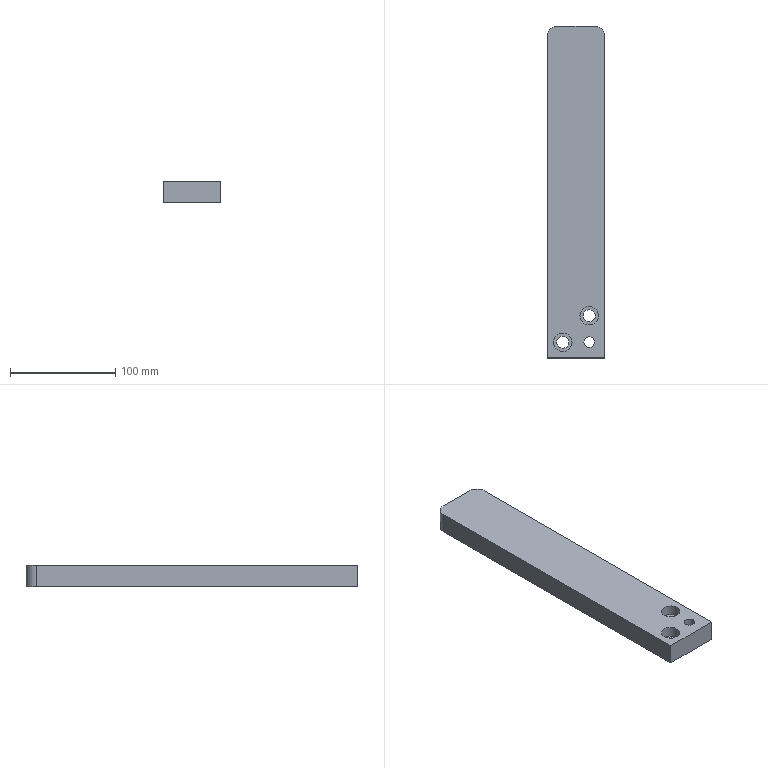Part | NX | features solid 2 | 1 solid | 15 faces | box 55 x 315 x 20 mm | volume 337183 mm3 | plane 8 | cylinder 7 | commonest cylinder face diameters 11.5 x2 17.5 x2 20 x2 10 x1
STEP:
#1=CARTESIAN_POINT('',(55.,25.,-20.));
#2=VERTEX_POINT('',#1);
#3=CARTESIAN_POINT('',(55.,25.,-40.));
#4=VERTEX_POINT('',#3);
#5=CARTESIAN_POINT('',(55.,25.,-20.));
#6=DIRECTION('',(0.,0.,-1.));
#7=VECTOR('',#6,1000.);
#8=LINE('',#5,#7);
#9=EDGE_CURVE('',#2,#4,#8,.T.);
#10=ORIENTED_EDGE('',*,*,#9,.T.);
#11=CARTESIAN_POINT('',(110.,25.,-40.));
#12=VERTEX_POINT('',#11);
#13=CARTESIAN_POINT('',(60.,25.,-40.));
#14=DIRECTION('',(-1.,0.,0.));
#15=VECTOR('',#14,1000.);
#16=LINE('',#13,#15);
#17=EDGE_CURVE('',#4,#12,#16,.F.);
#18=ORIENTED_EDGE('',*,*,#17,.T.);
#19=CARTESIAN_POINT('',(110.,25.,-20.));
#20=VERTEX_POINT('',#19);
#21=CARTESIAN_POINT('',(110.,25.,-20.));
#22=DIRECTION('',(0.,0.,1.));
#23=VECTOR('',#22,1000.);
#24=LINE('',#21,#23);
#25=EDGE_CURVE('',#20,#12,#24,.F.);
#26=ORIENTED_EDGE('',*,*,#25,.F.);
#27=CARTESIAN_POINT('',(60.,25.,-20.));
#28=DIRECTION('',(-1.,0.,0.));
#29=VECTOR('',#28,1000.);
#30=LINE('',#27,#29);
#31=EDGE_CURVE('',#2,#20,#30,.F.);
#32=ORIENTED_EDGE('',*,*,#31,.F.);
#33=EDGE_LOOP('',(#10,#18,#26,#32));
#34=FACE_BOUND('',#33,.T.);
#35=CARTESIAN_POINT('',(60.,25.,-20.));
#36=DIRECTION('',(0.,1.,0.));
#37=DIRECTION('',(1.,0.,0.));
#38=AXIS2_PLACEMENT_3D('',#35,#36,#37);
#39=PLANE('',#38);
#40=ADVANCED_FACE('',(#34),#39,.F.);
#41=CARTESIAN_POINT('',(100.,40.,-40.));
#42=VERTEX_POINT('',#41);
#43=CARTESIAN_POINT('',(95.,40.,-40.));
#44=DIRECTION('',(0.,0.,1.));
#45=DIRECTION('',(1.,0.,0.));
#46=AXIS2_PLACEMENT_3D('',#43,#44,#45);
#47=CIRCLE('',#46,5.);
#48=EDGE_CURVE('',#42,#42,#47,.T.);
#49=ORIENTED_EDGE('',*,*,#48,.T.);
#50=EDGE_LOOP('',(#49));
#51=FACE_BOUND('',#50,.T.);
#52=CARTESIAN_POINT('',(100.75,65.,-40.));
#53=VERTEX_POINT('',#52);
#54=CARTESIAN_POINT('',(95.,65.,-40.));
#55=DIRECTION('',(0.,0.,1.));
#56=DIRECTION('',(1.,0.,0.));
#57=AXIS2_PLACEMENT_3D('',#54,#55,#56);
#58=CIRCLE('',#57,5.75);
#59=EDGE_CURVE('',#53,#53,#58,.T.);
#60=ORIENTED_EDGE('',*,*,#59,.T.);
#61=EDGE_LOOP('',(#60));
#62=FACE_BOUND('',#61,.T.);
#63=CARTESIAN_POINT('',(75.75,40.,-40.));
#64=VERTEX_POINT('',#63);
#65=CARTESIAN_POINT('',(70.,40.,-40.));
#66=DIRECTION('',(0.,0.,1.));
#67=DIRECTION('',(1.,0.,0.));
#68=AXIS2_PLACEMENT_3D('',#65,#66,#67);
#69=CIRCLE('',#68,5.75);
#70=EDGE_CURVE('',#64,#64,#69,.T.);
#71=ORIENTED_EDGE('',*,*,#70,.T.);
#72=EDGE_LOOP('',(#71));
#73=FACE_BOUND('',#72,.T.);
#74=CARTESIAN_POINT('',(65.,340.,-40.));
#75=VERTEX_POINT('',#74);
#76=CARTESIAN_POINT('',(100.,340.,-40.));
#77=VERTEX_POINT('',#76);
#78=CARTESIAN_POINT('',(390.,340.,-40.));
#79=DIRECTION('',(1.,0.,0.));
#80=VECTOR('',#79,1000.);
#81=LINE('',#78,#80);
#82=EDGE_CURVE('',#75,#77,#81,.T.);
#83=ORIENTED_EDGE('',*,*,#82,.T.);
#84=CARTESIAN_POINT('',(110.,330.,-40.));
#85=VERTEX_POINT('',#84);
#86=CARTESIAN_POINT('',(100.,330.,-40.));
#87=DIRECTION('',(0.,0.,1.));
#88=DIRECTION('',(1.,0.,0.));
#89=AXIS2_PLACEMENT_3D('',#86,#87,#88);
#90=CIRCLE('',#89,10.);
#91=EDGE_CURVE('',#77,#85,#90,.F.);
#92=ORIENTED_EDGE('',*,*,#91,.T.);
#93=CARTESIAN_POINT('',(110.,120.,-40.));
#94=DIRECTION('',(0.,-1.,0.));
#95=VECTOR('',#94,1000.);
#96=LINE('',#93,#95);
#97=EDGE_CURVE('',#85,#12,#96,.T.);
#98=ORIENTED_EDGE('',*,*,#97,.T.);
#99=ORIENTED_EDGE('',*,*,#17,.F.);
#100=CARTESIAN_POINT('',(55.,330.,-40.));
#101=VERTEX_POINT('',#100);
#102=CARTESIAN_POINT('',(55.,120.,-40.));
#103=DIRECTION('',(0.,1.,0.));
#104=VECTOR('',#103,1000.);
#105=LINE('',#102,#104);
#106=EDGE_CURVE('',#101,#4,#105,.F.);
#107=ORIENTED_EDGE('',*,*,#106,.F.);
#108=CARTESIAN_POINT('',(65.,330.,-40.));
#109=DIRECTION('',(0.,0.,1.));
#110=DIRECTION('',(1.,0.,0.));
#111=AXIS2_PLACEMENT_3D('',#108,#109,#110);
#112=CIRCLE('',#111,10.);
#113=EDGE_CURVE('',#101,#75,#112,.F.);
#114=ORIENTED_EDGE('',*,*,#113,.T.);
#115=EDGE_LOOP('',(#83,#92,#98,#99,#107,#114));
#116=FACE_BOUND('',#115,.T.);
#117=CARTESIAN_POINT('',(60.,120.,-40.));
#118=DIRECTION('',(0.,0.,1.));
#119=DIRECTION('',(-1.,0.,0.));
#120=AXIS2_PLACEMENT_3D('',#117,#118,#119);
#121=PLANE('',#120);
#122=ADVANCED_FACE('',(#51,#62,#73,#116),#121,.F.);
#123=CARTESIAN_POINT('',(100.,40.,-20.));
#124=VERTEX_POINT('',#123);
#125=CARTESIAN_POINT('',(95.,40.,-20.));
#126=DIRECTION('',(0.,0.,1.));
#127=DIRECTION('',(1.,0.,0.));
#128=AXIS2_PLACEMENT_3D('',#125,#126,#127);
#129=CIRCLE('',#128,5.);
#130=EDGE_CURVE('',#124,#124,#129,.F.);
#131=ORIENTED_EDGE('',*,*,#130,.T.);
#132=EDGE_LOOP('',(#131));
#133=FACE_BOUND('',#132,.T.);
#134=CARTESIAN_POINT('',(103.75,65.,-20.));
#135=VERTEX_POINT('',#134);
#136=CARTESIAN_POINT('',(95.,65.,-20.));
#137=DIRECTION('',(0.,0.,1.));
#138=DIRECTION('',(1.,0.,0.));
#139=AXIS2_PLACEMENT_3D('',#136,#137,#138);
#140=CIRCLE('',#139,8.75);
#141=EDGE_CURVE('',#135,#135,#140,.F.);
#142=ORIENTED_EDGE('',*,*,#141,.T.);
#143=EDGE_LOOP('',(#142));
#144=FACE_BOUND('',#143,.T.);
#145=CARTESIAN_POINT('',(78.75,40.,-20.));
#146=VERTEX_POINT('',#145);
#147=CARTESIAN_POINT('',(70.,40.,-20.));
#148=DIRECTION('',(0.,0.,1.));
#149=DIRECTION('',(1.,0.,0.));
#150=AXIS2_PLACEMENT_3D('',#147,#148,#149);
#151=CIRCLE('',#150,8.75);
#152=EDGE_CURVE('',#146,#146,#151,.F.);
#153=ORIENTED_EDGE('',*,*,#152,.T.);
#154=EDGE_LOOP('',(#153));
#155=FACE_BOUND('',#154,.T.);
#156=CARTESIAN_POINT('',(110.,330.,-20.));
#157=VERTEX_POINT('',#156);
#158=CARTESIAN_POINT('',(110.,120.,-20.));
#159=DIRECTION('',(0.,-1.,0.));
#160=VECTOR('',#159,1000.);
#161=LINE('',#158,#160);
#162=EDGE_CURVE('',#157,#20,#161,.T.);
#163=ORIENTED_EDGE('',*,*,#162,.F.);
#164=CARTESIAN_POINT('',(100.,340.,-20.));
#165=VERTEX_POINT('',#164);
#166=CARTESIAN_POINT('',(100.,330.,-20.));
#167=DIRECTION('',(0.,0.,1.));
#168=DIRECTION('',(1.,0.,0.));
#169=AXIS2_PLACEMENT_3D('',#166,#167,#168);
#170=CIRCLE('',#169,10.);
#171=EDGE_CURVE('',#157,#165,#170,.T.);
#172=ORIENTED_EDGE('',*,*,#171,.T.);
#173=CARTESIAN_POINT('',(65.,340.,-20.));
#174=VERTEX_POINT('',#173);
#175=CARTESIAN_POINT('',(390.,340.,-20.));
#176=DIRECTION('',(1.,0.,0.));
#177=VECTOR('',#176,1000.);
#178=LINE('',#175,#177);
#179=EDGE_CURVE('',#174,#165,#178,.T.);
#180=ORIENTED_EDGE('',*,*,#179,.F.);
#181=CARTESIAN_POINT('',(55.,330.,-20.));
#182=VERTEX_POINT('',#181);
#183=CARTESIAN_POINT('',(65.,330.,-20.));
#184=DIRECTION('',(0.,0.,1.));
#185=DIRECTION('',(1.,0.,0.));
#186=AXIS2_PLACEMENT_3D('',#183,#184,#185);
#187=CIRCLE('',#186,10.);
#188=EDGE_CURVE('',#174,#182,#187,.T.);
#189=ORIENTED_EDGE('',*,*,#188,.T.);
#190=CARTESIAN_POINT('',(55.,120.,-20.));
#191=DIRECTION('',(0.,1.,0.));
#192=VECTOR('',#191,1000.);
#193=LINE('',#190,#192);
#194=EDGE_CURVE('',#182,#2,#193,.F.);
#195=ORIENTED_EDGE('',*,*,#194,.T.);
#196=ORIENTED_EDGE('',*,*,#31,.T.);
#197=EDGE_LOOP('',(#163,#172,#180,#189,#195,#196));
#198=FACE_BOUND('',#197,.T.);
#199=CARTESIAN_POINT('',(60.,120.,-20.));
#200=DIRECTION('',(0.,0.,1.));
#201=DIRECTION('',(-1.,0.,0.));
#202=AXIS2_PLACEMENT_3D('',#199,#200,#201);
#203=PLANE('',#202);
#204=ADVANCED_FACE('',(#133,#144,#155,#198),#203,.T.);
#205=ORIENTED_EDGE('',*,*,#97,.F.);
#206=CARTESIAN_POINT('',(110.,330.,-20.));
#207=DIRECTION('',(0.,0.,-1.));
#208=VECTOR('',#207,1000.);
#209=LINE('',#206,#208);
#210=EDGE_CURVE('',#85,#157,#209,.F.);
#211=ORIENTED_EDGE('',*,*,#210,.T.);
#212=ORIENTED_EDGE('',*,*,#162,.T.);
#213=ORIENTED_EDGE('',*,*,#25,.T.);
#214=EDGE_LOOP('',(#205,#211,#212,#213));
#215=FACE_BOUND('',#214,.T.);
#216=CARTESIAN_POINT('',(110.,120.,-20.));
#217=DIRECTION('',(1.,0.,0.));
#218=DIRECTION('',(0.,-1.,0.));
#219=AXIS2_PLACEMENT_3D('',#216,#217,#218);
#220=PLANE('',#219);
#221=ADVANCED_FACE('',(#215),#220,.T.);
#222=ORIENTED_EDGE('',*,*,#194,.F.);
#223=CARTESIAN_POINT('',(55.,330.,-20.));
#224=DIRECTION('',(0.,0.,1.));
#225=VECTOR('',#224,1000.);
#226=LINE('',#223,#225);
#227=EDGE_CURVE('',#182,#101,#226,.F.);
#228=ORIENTED_EDGE('',*,*,#227,.T.);
#229=ORIENTED_EDGE('',*,*,#106,.T.);
#230=ORIENTED_EDGE('',*,*,#9,.F.);
#231=EDGE_LOOP('',(#222,#228,#229,#230));
#232=FACE_BOUND('',#231,.T.);
#233=CARTESIAN_POINT('',(55.,120.,-20.));
#234=DIRECTION('',(1.,0.,0.));
#235=DIRECTION('',(0.,-1.,0.));
#236=AXIS2_PLACEMENT_3D('',#233,#234,#235);
#237=PLANE('',#236);
#238=ADVANCED_FACE('',(#232),#237,.F.);
#239=ORIENTED_EDGE('',*,*,#179,.T.);
#240=CARTESIAN_POINT('',(100.,340.,15.));
#241=DIRECTION('',(0.,0.,-1.));
#242=VECTOR('',#241,1000.);
#243=LINE('',#240,#242);
#244=EDGE_CURVE('',#165,#77,#243,.T.);
#245=ORIENTED_EDGE('',*,*,#244,.T.);
#246=ORIENTED_EDGE('',*,*,#82,.F.);
#247=CARTESIAN_POINT('',(65.,340.,15.));
#248=DIRECTION('',(0.,0.,-1.));
#249=VECTOR('',#248,1000.);
#250=LINE('',#247,#249);
#251=EDGE_CURVE('',#75,#174,#250,.F.);
#252=ORIENTED_EDGE('',*,*,#251,.T.);
#253=EDGE_LOOP('',(#239,#245,#246,#252));
#254=FACE_BOUND('',#253,.T.);
#255=CARTESIAN_POINT('',(390.,340.,15.));
#256=DIRECTION('',(0.,1.,0.));
#257=DIRECTION('',(0.,0.,1.));
#258=AXIS2_PLACEMENT_3D('',#255,#256,#257);
#259=PLANE('',#258);
#260=ADVANCED_FACE('',(#254),#259,.T.);
#261=CARTESIAN_POINT('',(64.25,40.,-30.));
#262=VERTEX_POINT('',#261);
#263=CARTESIAN_POINT('',(70.,40.,-30.));
#264=DIRECTION('',(0.,0.,-1.));
#265=DIRECTION('',(-1.,0.,0.));
#266=AXIS2_PLACEMENT_3D('',#263,#264,#265);
#267=CIRCLE('',#266,5.75);
#268=EDGE_CURVE('',#262,#262,#267,.T.);
#269=ORIENTED_EDGE('',*,*,#268,.F.);
#270=EDGE_LOOP('',(#269));
#271=FACE_BOUND('',#270,.T.);
#272=ORIENTED_EDGE('',*,*,#70,.F.);
#273=EDGE_LOOP('',(#272));
#274=FACE_BOUND('',#273,.T.);
#275=CARTESIAN_POINT('',(70.,40.,-115.));
#276=DIRECTION('',(0.,0.,-1.));
#277=DIRECTION('',(-1.,0.,0.));
#278=AXIS2_PLACEMENT_3D('',#275,#276,#277);
#279=CYLINDRICAL_SURFACE('',#278,5.75);
#280=ADVANCED_FACE('',(#271,#274),#279,.F.);
#281=ORIENTED_EDGE('',*,*,#268,.T.);
#282=EDGE_LOOP('',(#281));
#283=FACE_BOUND('',#282,.T.);
#284=CARTESIAN_POINT('',(61.25,40.,-30.));
#285=VERTEX_POINT('',#284);
#286=CARTESIAN_POINT('',(70.,40.,-30.));
#287=DIRECTION('',(0.,0.,-1.));
#288=DIRECTION('',(-1.,0.,0.));
#289=AXIS2_PLACEMENT_3D('',#286,#287,#288);
#290=CIRCLE('',#289,8.75);
#291=EDGE_CURVE('',#285,#285,#290,.T.);
#292=ORIENTED_EDGE('',*,*,#291,.F.);
#293=EDGE_LOOP('',(#292));
#294=FACE_BOUND('',#293,.T.);
#295=CARTESIAN_POINT('',(70.,40.,-30.));
#296=DIRECTION('',(0.,0.,-1.));
#297=DIRECTION('',(-1.,0.,0.));
#298=AXIS2_PLACEMENT_3D('',#295,#296,#297);
#299=PLANE('',#298);
#300=ADVANCED_FACE('',(#283,#294),#299,.F.);
#301=ORIENTED_EDGE('',*,*,#291,.T.);
#302=EDGE_LOOP('',(#301));
#303=FACE_BOUND('',#302,.T.);
#304=ORIENTED_EDGE('',*,*,#152,.F.);
#305=EDGE_LOOP('',(#304));
#306=FACE_BOUND('',#305,.T.);
#307=CARTESIAN_POINT('',(70.,40.,-15.));
#308=DIRECTION('',(0.,0.,-1.));
#309=DIRECTION('',(-1.,0.,0.));
#310=AXIS2_PLACEMENT_3D('',#307,#308,#309);
#311=CYLINDRICAL_SURFACE('',#310,8.75);
#312=ADVANCED_FACE('',(#303,#306),#311,.F.);
#313=CARTESIAN_POINT('',(89.25,65.,-30.));
#314=VERTEX_POINT('',#313);
#315=CARTESIAN_POINT('',(95.,65.,-30.));
#316=DIRECTION('',(0.,0.,-1.));
#317=DIRECTION('',(-1.,0.,0.));
#318=AXIS2_PLACEMENT_3D('',#315,#316,#317);
#319=CIRCLE('',#318,5.75);
#320=EDGE_CURVE('',#314,#314,#319,.T.);
#321=ORIENTED_EDGE('',*,*,#320,.F.);
#322=EDGE_LOOP('',(#321));
#323=FACE_BOUND('',#322,.T.);
#324=ORIENTED_EDGE('',*,*,#59,.F.);
#325=EDGE_LOOP('',(#324));
#326=FACE_BOUND('',#325,.T.);
#327=CARTESIAN_POINT('',(95.,65.,-115.));
#328=DIRECTION('',(0.,0.,-1.));
#329=DIRECTION('',(-1.,0.,0.));
#330=AXIS2_PLACEMENT_3D('',#327,#328,#329);
#331=CYLINDRICAL_SURFACE('',#330,5.75);
#332=ADVANCED_FACE('',(#323,#326),#331,.F.);
#333=ORIENTED_EDGE('',*,*,#320,.T.);
#334=EDGE_LOOP('',(#333));
#335=FACE_BOUND('',#334,.T.);
#336=CARTESIAN_POINT('',(86.25,65.,-30.));
#337=VERTEX_POINT('',#336);
#338=CARTESIAN_POINT('',(95.,65.,-30.));
#339=DIRECTION('',(0.,0.,-1.));
#340=DIRECTION('',(-1.,0.,0.));
#341=AXIS2_PLACEMENT_3D('',#338,#339,#340);
#342=CIRCLE('',#341,8.75);
#343=EDGE_CURVE('',#337,#337,#342,.T.);
#344=ORIENTED_EDGE('',*,*,#343,.F.);
#345=EDGE_LOOP('',(#344));
#346=FACE_BOUND('',#345,.T.);
#347=CARTESIAN_POINT('',(95.,65.,-30.));
#348=DIRECTION('',(0.,0.,-1.));
#349=DIRECTION('',(-1.,0.,0.));
#350=AXIS2_PLACEMENT_3D('',#347,#348,#349);
#351=PLANE('',#350);
#352=ADVANCED_FACE('',(#335,#346),#351,.F.);
#353=ORIENTED_EDGE('',*,*,#343,.T.);
#354=EDGE_LOOP('',(#353));
#355=FACE_BOUND('',#354,.T.);
#356=ORIENTED_EDGE('',*,*,#141,.F.);
#357=EDGE_LOOP('',(#356));
#358=FACE_BOUND('',#357,.T.);
#359=CARTESIAN_POINT('',(95.,65.,-15.));
#360=DIRECTION('',(0.,0.,-1.));
#361=DIRECTION('',(-1.,0.,0.));
#362=AXIS2_PLACEMENT_3D('',#359,#360,#361);
#363=CYLINDRICAL_SURFACE('',#362,8.75);
#364=ADVANCED_FACE('',(#355,#358),#363,.F.);
#365=ORIENTED_EDGE('',*,*,#130,.F.);
#366=EDGE_LOOP('',(#365));
#367=FACE_BOUND('',#366,.T.);
#368=ORIENTED_EDGE('',*,*,#48,.F.);
#369=EDGE_LOOP('',(#368));
#370=FACE_BOUND('',#369,.T.);
#371=CARTESIAN_POINT('',(95.,40.,-15.));
#372=DIRECTION('',(0.,0.,-1.));
#373=DIRECTION('',(-1.,0.,0.));
#374=AXIS2_PLACEMENT_3D('',#371,#372,#373);
#375=CYLINDRICAL_SURFACE('',#374,5.);
#376=ADVANCED_FACE('',(#367,#370),#375,.F.);
#377=ORIENTED_EDGE('',*,*,#171,.F.);
#378=ORIENTED_EDGE('',*,*,#210,.F.);
#379=ORIENTED_EDGE('',*,*,#91,.F.);
#380=ORIENTED_EDGE('',*,*,#244,.F.);
#381=EDGE_LOOP('',(#377,#378,#379,#380));
#382=FACE_BOUND('',#381,.T.);
#383=CARTESIAN_POINT('',(100.,330.,15.));
#384=DIRECTION('',(0.,0.,-1.));
#385=DIRECTION('',(-1.,0.,0.));
#386=AXIS2_PLACEMENT_3D('',#383,#384,#385);
#387=CYLINDRICAL_SURFACE('',#386,10.);
#388=ADVANCED_FACE('',(#382),#387,.T.);
#389=ORIENTED_EDGE('',*,*,#113,.F.);
#390=ORIENTED_EDGE('',*,*,#227,.F.);
#391=ORIENTED_EDGE('',*,*,#188,.F.);
#392=ORIENTED_EDGE('',*,*,#251,.F.);
#393=EDGE_LOOP('',(#389,#390,#391,#392));
#394=FACE_BOUND('',#393,.T.);
#395=CARTESIAN_POINT('',(65.,330.,15.));
#396=DIRECTION('',(0.,0.,-1.));
#397=DIRECTION('',(-1.,0.,0.));
#398=AXIS2_PLACEMENT_3D('',#395,#396,#397);
#399=CYLINDRICAL_SURFACE('',#398,10.);
#400=ADVANCED_FACE('',(#394),#399,.T.);
#401=CLOSED_SHELL('',(#40,#122,#204,#221,#238,#260,#280,#300,#312,#332,#352,#364,#376,#388,#400));
#402=MANIFOLD_SOLID_BREP('',#401);
#403=(LENGTH_UNIT()NAMED_UNIT(*)SI_UNIT(.MILLI.,.METRE.));
#404=UNCERTAINTY_MEASURE_WITH_UNIT(LENGTH_MEASURE(0.00001),#403,'','');
#405=(NAMED_UNIT(*)PLANE_ANGLE_UNIT()SI_UNIT($,.RADIAN.));
#406=(NAMED_UNIT(*)SI_UNIT($,.STERADIAN.)SOLID_ANGLE_UNIT());
#407=(GEOMETRIC_REPRESENTATION_CONTEXT(3)GLOBAL_UNCERTAINTY_ASSIGNED_CONTEXT((#404))GLOBAL_UNIT_ASSIGNED_CONTEXT((#403,#405,#406))REPRESENTATION_CONTEXT('',''));
#408=ADVANCED_BREP_SHAPE_REPRESENTATION('',(#402),#407);